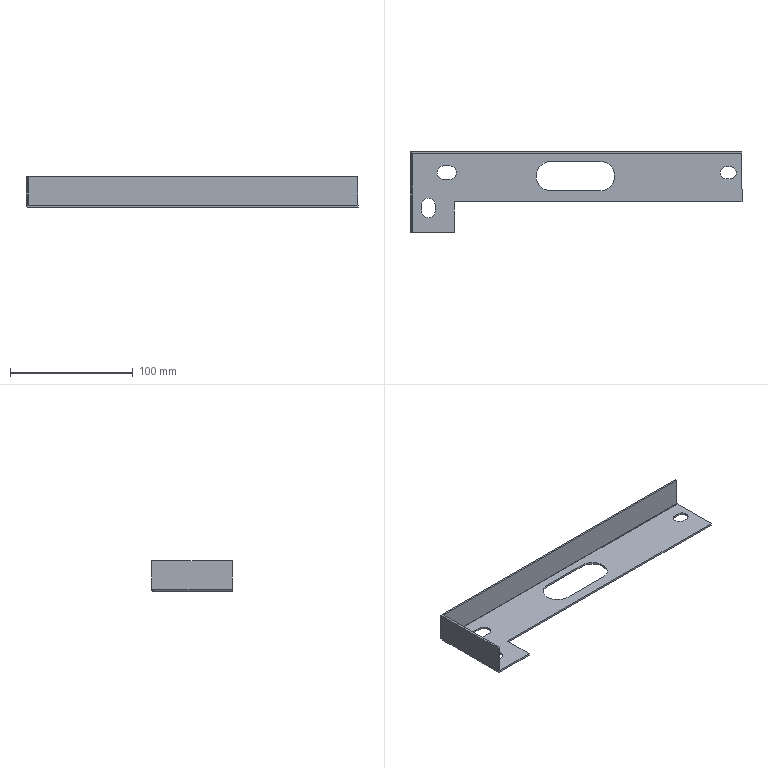Part | 1 solid | 44 faces | box 271 x 66 x 25 mm | volume 26895 mm3 | plane 29 | cylinder 15 | commonest cylinder face diameters 11 x5 10 x3 24 x3 0.4 x2 3.4 x2
STEP:
#1=CARTESIAN_POINT('',(130.8,15.8,-1.5));
#2=VERTEX_POINT('',#1);
#3=CARTESIAN_POINT('',(125.8,20.8,-1.5));
#4=VERTEX_POINT('',#3);
#5=CARTESIAN_POINT('',(125.8,15.8,-1.5));
#6=DIRECTION('',(0.,0.,1.));
#7=DIRECTION('',(1.,0.,0.));
#8=AXIS2_PLACEMENT_3D('',#5,#6,#7);
#9=CIRCLE('',#8,5.);
#10=EDGE_CURVE('',#2,#4,#9,.T.);
#11=ORIENTED_EDGE('',*,*,#10,.F.);
#12=CARTESIAN_POINT('',(130.8,15.8,0.));
#13=VERTEX_POINT('',#12);
#14=CARTESIAN_POINT('',(130.8,15.8,-10.));
#15=DIRECTION('',(0.,0.,1.));
#16=VECTOR('',#15,1000.);
#17=LINE('',#14,#16);
#18=EDGE_CURVE('',#2,#13,#17,.T.);
#19=ORIENTED_EDGE('',*,*,#18,.T.);
#20=CARTESIAN_POINT('',(125.8,20.8,0.));
#21=VERTEX_POINT('',#20);
#22=CARTESIAN_POINT('',(125.8,15.8,0.));
#23=DIRECTION('',(0.,0.,1.));
#24=DIRECTION('',(1.,0.,0.));
#25=AXIS2_PLACEMENT_3D('',#22,#23,#24);
#26=CIRCLE('',#25,5.);
#27=EDGE_CURVE('',#13,#21,#26,.T.);
#28=ORIENTED_EDGE('',*,*,#27,.T.);
#29=CARTESIAN_POINT('',(125.8,20.8,-10.));
#30=DIRECTION('',(0.,0.,1.));
#31=VECTOR('',#30,1000.);
#32=LINE('',#29,#31);
#33=EDGE_CURVE('',#4,#21,#32,.T.);
#34=ORIENTED_EDGE('',*,*,#33,.F.);
#35=EDGE_LOOP('',(#11,#19,#28,#34));
#36=FACE_OUTER_BOUND('',#35,.T.);
#37=CARTESIAN_POINT('',(125.8,15.8,-10.));
#38=DIRECTION('',(0.,0.,1.));
#39=DIRECTION('',(1.,0.,0.));
#40=AXIS2_PLACEMENT_3D('',#37,#38,#39);
#41=CYLINDRICAL_SURFACE('',#40,5.);
#42=ADVANCED_FACE('',(#36),#41,.F.);
#43=CARTESIAN_POINT('',(-97.5,15.8,-1.5));
#44=VERTEX_POINT('',#43);
#45=CARTESIAN_POINT('',(-103.,21.3,-1.5));
#46=VERTEX_POINT('',#45);
#47=CARTESIAN_POINT('',(-103.,15.8,-1.5));
#48=DIRECTION('',(0.,0.,1.));
#49=DIRECTION('',(1.,0.,0.));
#50=AXIS2_PLACEMENT_3D('',#47,#48,#49);
#51=CIRCLE('',#50,5.5);
#52=EDGE_CURVE('',#44,#46,#51,.T.);
#53=ORIENTED_EDGE('',*,*,#52,.F.);
#54=CARTESIAN_POINT('',(-97.5,15.8,0.));
#55=VERTEX_POINT('',#54);
#56=CARTESIAN_POINT('',(-97.5,15.8,-10.));
#57=DIRECTION('',(0.,0.,1.));
#58=VECTOR('',#57,1000.);
#59=LINE('',#56,#58);
#60=EDGE_CURVE('',#44,#55,#59,.T.);
#61=ORIENTED_EDGE('',*,*,#60,.T.);
#62=CARTESIAN_POINT('',(-103.,21.3,0.));
#63=VERTEX_POINT('',#62);
#64=CARTESIAN_POINT('',(-103.,15.8,0.));
#65=DIRECTION('',(0.,0.,1.));
#66=DIRECTION('',(1.,0.,0.));
#67=AXIS2_PLACEMENT_3D('',#64,#65,#66);
#68=CIRCLE('',#67,5.5);
#69=EDGE_CURVE('',#55,#63,#68,.T.);
#70=ORIENTED_EDGE('',*,*,#69,.T.);
#71=CARTESIAN_POINT('',(-103.,21.3,-10.));
#72=DIRECTION('',(0.,0.,1.));
#73=VECTOR('',#72,1000.);
#74=LINE('',#71,#73);
#75=EDGE_CURVE('',#46,#63,#74,.T.);
#76=ORIENTED_EDGE('',*,*,#75,.F.);
#77=EDGE_LOOP('',(#53,#61,#70,#76));
#78=FACE_OUTER_BOUND('',#77,.T.);
#79=CARTESIAN_POINT('',(-103.,15.8,-10.));
#80=DIRECTION('',(0.,0.,1.));
#81=DIRECTION('',(1.,0.,0.));
#82=AXIS2_PLACEMENT_3D('',#79,#80,#81);
#83=CYLINDRICAL_SURFACE('',#82,5.5);
#84=ADVANCED_FACE('',(#78),#83,.F.);
#85=CARTESIAN_POINT('',(31.5,13.,-1.5));
#86=VERTEX_POINT('',#85);
#87=CARTESIAN_POINT('',(19.5,25.,-1.5));
#88=VERTEX_POINT('',#87);
#89=CARTESIAN_POINT('',(19.5,13.,-1.5));
#90=DIRECTION('',(0.,0.,1.));
#91=DIRECTION('',(1.,0.,0.));
#92=AXIS2_PLACEMENT_3D('',#89,#90,#91);
#93=CIRCLE('',#92,12.);
#94=EDGE_CURVE('',#86,#88,#93,.T.);
#95=ORIENTED_EDGE('',*,*,#94,.F.);
#96=CARTESIAN_POINT('',(31.5,13.,0.));
#97=VERTEX_POINT('',#96);
#98=CARTESIAN_POINT('',(31.5,13.,-10.));
#99=DIRECTION('',(0.,0.,1.));
#100=VECTOR('',#99,1000.);
#101=LINE('',#98,#100);
#102=EDGE_CURVE('',#86,#97,#101,.T.);
#103=ORIENTED_EDGE('',*,*,#102,.T.);
#104=CARTESIAN_POINT('',(19.5,25.,0.));
#105=VERTEX_POINT('',#104);
#106=CARTESIAN_POINT('',(19.5,13.,0.));
#107=DIRECTION('',(0.,0.,1.));
#108=DIRECTION('',(1.,0.,0.));
#109=AXIS2_PLACEMENT_3D('',#106,#107,#108);
#110=CIRCLE('',#109,12.);
#111=EDGE_CURVE('',#97,#105,#110,.T.);
#112=ORIENTED_EDGE('',*,*,#111,.T.);
#113=CARTESIAN_POINT('',(19.5,25.,-10.));
#114=DIRECTION('',(0.,0.,1.));
#115=VECTOR('',#114,1000.);
#116=LINE('',#113,#115);
#117=EDGE_CURVE('',#88,#105,#116,.T.);
#118=ORIENTED_EDGE('',*,*,#117,.F.);
#119=EDGE_LOOP('',(#95,#103,#112,#118));
#120=FACE_OUTER_BOUND('',#119,.T.);
#121=CARTESIAN_POINT('',(19.5,13.,-10.));
#122=DIRECTION('',(0.,0.,1.));
#123=DIRECTION('',(1.,0.,0.));
#124=AXIS2_PLACEMENT_3D('',#121,#122,#123);
#125=CYLINDRICAL_SURFACE('',#124,12.);
#126=ADVANCED_FACE('',(#120),#125,.F.);
#127=CARTESIAN_POINT('',(-135.5,31.3,0.2));
#128=VERTEX_POINT('',#127);
#129=CARTESIAN_POINT('',(-134.,31.3,0.2));
#130=VERTEX_POINT('',#129);
#131=CARTESIAN_POINT('',(-135.5,31.3,0.2));
#132=DIRECTION('',(1.,0.,0.));
#133=VECTOR('',#132,1000.);
#134=LINE('',#131,#133);
#135=EDGE_CURVE('',#128,#130,#134,.T.);
#136=ORIENTED_EDGE('',*,*,#135,.F.);
#137=CARTESIAN_POINT('',(-135.5,33.,0.2));
#138=VERTEX_POINT('',#137);
#139=CARTESIAN_POINT('',(-135.5,33.,0.2));
#140=DIRECTION('',(0.,1.,0.));
#141=VECTOR('',#140,1000.);
#142=LINE('',#139,#141);
#143=EDGE_CURVE('',#128,#138,#142,.T.);
#144=ORIENTED_EDGE('',*,*,#143,.T.);
#145=CARTESIAN_POINT('',(-134.,33.,0.2));
#146=VERTEX_POINT('',#145);
#147=CARTESIAN_POINT('',(-135.5,33.,0.2));
#148=DIRECTION('',(-1.,0.,0.));
#149=VECTOR('',#148,1000.);
#150=LINE('',#147,#149);
#151=EDGE_CURVE('',#146,#138,#150,.T.);
#152=ORIENTED_EDGE('',*,*,#151,.F.);
#153=CARTESIAN_POINT('',(-134.,33.,0.2));
#154=DIRECTION('',(0.,-1.,0.));
#155=VECTOR('',#154,1000.);
#156=LINE('',#153,#155);
#157=EDGE_CURVE('',#146,#130,#156,.T.);
#158=ORIENTED_EDGE('',*,*,#157,.T.);
#159=EDGE_LOOP('',(#136,#144,#152,#158));
#160=FACE_OUTER_BOUND('',#159,.T.);
#161=CARTESIAN_POINT('',(0.,0.,0.2));
#162=DIRECTION('',(0.,0.,-1.));
#163=DIRECTION('',(-1.,0.,0.));
#164=AXIS2_PLACEMENT_3D('',#161,#162,#163);
#165=PLANE('',#164);
#166=ADVANCED_FACE('',(#160),#165,.T.);
#167=CARTESIAN_POINT('',(-135.5,-33.,0.2));
#168=VERTEX_POINT('',#167);
#169=CARTESIAN_POINT('',(-135.5,33.,0.2));
#170=DIRECTION('',(0.,1.,0.));
#171=VECTOR('',#170,1000.);
#172=LINE('',#169,#171);
#173=EDGE_CURVE('',#168,#128,#172,.T.);
#174=ORIENTED_EDGE('',*,*,#173,.T.);
#175=CARTESIAN_POINT('',(-133.8,31.3,-1.5));
#176=VERTEX_POINT('',#175);
#177=CARTESIAN_POINT('',(-133.8,31.3,0.2));
#178=DIRECTION('',(0.,-1.,0.));
#179=DIRECTION('',(0.,0.,1.));
#180=AXIS2_PLACEMENT_3D('',#177,#178,#179);
#181=CIRCLE('',#180,1.7);
#182=EDGE_CURVE('',#128,#176,#181,.T.);
#183=ORIENTED_EDGE('',*,*,#182,.T.);
#184=CARTESIAN_POINT('',(-133.8,-33.,-1.5));
#185=VERTEX_POINT('',#184);
#186=CARTESIAN_POINT('',(-133.8,-33.,-1.5));
#187=DIRECTION('',(0.,1.,0.));
#188=VECTOR('',#187,1000.);
#189=LINE('',#186,#188);
#190=EDGE_CURVE('',#185,#176,#189,.T.);
#191=ORIENTED_EDGE('',*,*,#190,.F.);
#192=CARTESIAN_POINT('',(-133.8,-33.,0.2));
#193=DIRECTION('',(0.,-1.,0.));
#194=DIRECTION('',(0.,0.,-1.));
#195=AXIS2_PLACEMENT_3D('',#192,#193,#194);
#196=CIRCLE('',#195,1.7);
#197=EDGE_CURVE('',#168,#185,#196,.T.);
#198=ORIENTED_EDGE('',*,*,#197,.F.);
#199=EDGE_LOOP('',(#174,#183,#191,#198));
#200=FACE_OUTER_BOUND('',#199,.T.);
#201=CARTESIAN_POINT('',(-133.8,-33.,0.2));
#202=DIRECTION('',(0.,-1.,0.));
#203=DIRECTION('',(-1.,0.,0.));
#204=AXIS2_PLACEMENT_3D('',#201,#202,#203);
#205=CYLINDRICAL_SURFACE('',#204,1.7);
#206=ADVANCED_FACE('',(#200),#205,.T.);
#207=CARTESIAN_POINT('',(122.8,20.8,-1.5));
#208=VERTEX_POINT('',#207);
#209=CARTESIAN_POINT('',(0.,20.8,-1.5));
#210=DIRECTION('',(-1.,0.,0.));
#211=VECTOR('',#210,1000.);
#212=LINE('',#209,#211);
#213=EDGE_CURVE('',#4,#208,#212,.T.);
#214=ORIENTED_EDGE('',*,*,#213,.T.);
#215=CARTESIAN_POINT('',(122.8,10.8,-1.5));
#216=VERTEX_POINT('',#215);
#217=CARTESIAN_POINT('',(122.8,15.8,-1.5));
#218=DIRECTION('',(0.,0.,1.));
#219=DIRECTION('',(1.,0.,0.));
#220=AXIS2_PLACEMENT_3D('',#217,#218,#219);
#221=CIRCLE('',#220,5.);
#222=EDGE_CURVE('',#208,#216,#221,.T.);
#223=ORIENTED_EDGE('',*,*,#222,.T.);
#224=CARTESIAN_POINT('',(125.8,10.8,-1.5));
#225=VERTEX_POINT('',#224);
#226=CARTESIAN_POINT('',(0.,10.8,-1.5));
#227=DIRECTION('',(1.,0.,0.));
#228=VECTOR('',#227,1000.);
#229=LINE('',#226,#228);
#230=EDGE_CURVE('',#216,#225,#229,.T.);
#231=ORIENTED_EDGE('',*,*,#230,.T.);
#232=CARTESIAN_POINT('',(125.8,15.8,-1.5));
#233=DIRECTION('',(0.,0.,1.));
#234=DIRECTION('',(1.,0.,0.));
#235=AXIS2_PLACEMENT_3D('',#232,#233,#234);
#236=CIRCLE('',#235,5.);
#237=EDGE_CURVE('',#225,#2,#236,.T.);
#238=ORIENTED_EDGE('',*,*,#237,.T.);
#239=ORIENTED_EDGE('',*,*,#10,.T.);
#240=EDGE_LOOP('',(#214,#223,#231,#238,#239));
#241=FACE_BOUND('',#240,.T.);
#242=CARTESIAN_POINT('',(-108.,21.3,-1.5));
#243=VERTEX_POINT('',#242);
#244=CARTESIAN_POINT('',(0.,21.3,-1.5));
#245=DIRECTION('',(-1.,0.,0.));
#246=VECTOR('',#245,1000.);
#247=LINE('',#244,#246);
#248=EDGE_CURVE('',#46,#243,#247,.T.);
#249=ORIENTED_EDGE('',*,*,#248,.T.);
#250=CARTESIAN_POINT('',(-108.,10.3,-1.5));
#251=VERTEX_POINT('',#250);
#252=CARTESIAN_POINT('',(-108.,15.8,-1.5));
#253=DIRECTION('',(0.,0.,1.));
#254=DIRECTION('',(1.,0.,0.));
#255=AXIS2_PLACEMENT_3D('',#252,#253,#254);
#256=CIRCLE('',#255,5.5);
#257=EDGE_CURVE('',#243,#251,#256,.T.);
#258=ORIENTED_EDGE('',*,*,#257,.T.);
#259=CARTESIAN_POINT('',(-103.,10.3,-1.5));
#260=VERTEX_POINT('',#259);
#261=CARTESIAN_POINT('',(0.,10.3,-1.5));
#262=DIRECTION('',(1.,0.,0.));
#263=VECTOR('',#262,1000.);
#264=LINE('',#261,#263);
#265=EDGE_CURVE('',#251,#260,#264,.T.);
#266=ORIENTED_EDGE('',*,*,#265,.T.);
#267=CARTESIAN_POINT('',(-103.,15.8,-1.5));
#268=DIRECTION('',(0.,0.,1.));
#269=DIRECTION('',(1.,0.,0.));
#270=AXIS2_PLACEMENT_3D('',#267,#268,#269);
#271=CIRCLE('',#270,5.5);
#272=EDGE_CURVE('',#260,#44,#271,.T.);
#273=ORIENTED_EDGE('',*,*,#272,.T.);
#274=ORIENTED_EDGE('',*,*,#52,.T.);
#275=EDGE_LOOP('',(#249,#258,#266,#273,#274));
#276=FACE_BOUND('',#275,.T.);
#277=CARTESIAN_POINT('',(-20.5,25.,-1.5));
#278=VERTEX_POINT('',#277);
#279=CARTESIAN_POINT('',(0.,25.,-1.5));
#280=DIRECTION('',(-1.,0.,0.));
#281=VECTOR('',#280,1000.);
#282=LINE('',#279,#281);
#283=EDGE_CURVE('',#88,#278,#282,.T.);
#284=ORIENTED_EDGE('',*,*,#283,.T.);
#285=CARTESIAN_POINT('',(-20.5,1.,-1.5));
#286=VERTEX_POINT('',#285);
#287=CARTESIAN_POINT('',(-20.5,13.,-1.5));
#288=DIRECTION('',(0.,0.,1.));
#289=DIRECTION('',(1.,0.,0.));
#290=AXIS2_PLACEMENT_3D('',#287,#288,#289);
#291=CIRCLE('',#290,12.);
#292=EDGE_CURVE('',#278,#286,#291,.T.);
#293=ORIENTED_EDGE('',*,*,#292,.T.);
#294=CARTESIAN_POINT('',(19.5,1.,-1.5));
#295=VERTEX_POINT('',#294);
#296=CARTESIAN_POINT('',(0.,1.,-1.5));
#297=DIRECTION('',(1.,0.,0.));
#298=VECTOR('',#297,1000.);
#299=LINE('',#296,#298);
#300=EDGE_CURVE('',#286,#295,#299,.T.);
#301=ORIENTED_EDGE('',*,*,#300,.T.);
#302=CARTESIAN_POINT('',(19.5,13.,-1.5));
#303=DIRECTION('',(0.,0.,1.));
#304=DIRECTION('',(1.,0.,0.));
#305=AXIS2_PLACEMENT_3D('',#302,#303,#304);
#306=CIRCLE('',#305,12.);
#307=EDGE_CURVE('',#295,#86,#306,.T.);
#308=ORIENTED_EDGE('',*,*,#307,.T.);
#309=ORIENTED_EDGE('',*,*,#94,.T.);
#310=EDGE_LOOP('',(#284,#293,#301,#308,#309));
#311=FACE_BOUND('',#310,.T.);
#312=CARTESIAN_POINT('',(-115.,-15.5,-1.5));
#313=VERTEX_POINT('',#312);
#314=CARTESIAN_POINT('',(-115.,-10.5,-1.5));
#315=VERTEX_POINT('',#314);
#316=CARTESIAN_POINT('',(-115.,0.,-1.5));
#317=DIRECTION('',(0.,1.,0.));
#318=VECTOR('',#317,1000.);
#319=LINE('',#316,#318);
#320=EDGE_CURVE('',#313,#315,#319,.T.);
#321=ORIENTED_EDGE('',*,*,#320,.T.);
#322=CARTESIAN_POINT('',(-126.,-10.5,-1.5));
#323=VERTEX_POINT('',#322);
#324=CARTESIAN_POINT('',(-120.5,-10.5,-1.5));
#325=DIRECTION('',(0.,0.,1.));
#326=DIRECTION('',(1.,0.,0.));
#327=AXIS2_PLACEMENT_3D('',#324,#325,#326);
#328=CIRCLE('',#327,5.5);
#329=EDGE_CURVE('',#315,#323,#328,.T.);
#330=ORIENTED_EDGE('',*,*,#329,.T.);
#331=CARTESIAN_POINT('',(-126.,-15.5,-1.5));
#332=VERTEX_POINT('',#331);
#333=CARTESIAN_POINT('',(-126.,0.,-1.5));
#334=DIRECTION('',(0.,-1.,0.));
#335=VECTOR('',#334,1000.);
#336=LINE('',#333,#335);
#337=EDGE_CURVE('',#323,#332,#336,.T.);
#338=ORIENTED_EDGE('',*,*,#337,.T.);
#339=CARTESIAN_POINT('',(-120.5,-15.5,-1.5));
#340=DIRECTION('',(0.,0.,1.));
#341=DIRECTION('',(1.,0.,0.));
#342=AXIS2_PLACEMENT_3D('',#339,#340,#341);
#343=CIRCLE('',#342,5.5);
#344=EDGE_CURVE('',#332,#313,#343,.T.);
#345=ORIENTED_EDGE('',*,*,#344,.T.);
#346=EDGE_LOOP('',(#321,#330,#338,#345));
#347=FACE_BOUND('',#346,.T.);
#348=CARTESIAN_POINT('',(135.5,-8.,-1.5));
#349=VERTEX_POINT('',#348);
#350=CARTESIAN_POINT('',(135.5,31.3,-1.5));
#351=VERTEX_POINT('',#350);
#352=CARTESIAN_POINT('',(135.5,33.,-1.5));
#353=DIRECTION('',(0.,1.,0.));
#354=VECTOR('',#353,1000.);
#355=LINE('',#352,#354);
#356=EDGE_CURVE('',#349,#351,#355,.T.);
#357=ORIENTED_EDGE('',*,*,#356,.F.);
#358=CARTESIAN_POINT('',(-99.5,-8.,-1.5));
#359=VERTEX_POINT('',#358);
#360=CARTESIAN_POINT('',(0.,-8.,-1.5));
#361=DIRECTION('',(-1.,0.,0.));
#362=VECTOR('',#361,1000.);
#363=LINE('',#360,#362);
#364=EDGE_CURVE('',#349,#359,#363,.T.);
#365=ORIENTED_EDGE('',*,*,#364,.T.);
#366=CARTESIAN_POINT('',(-99.5,-33.,-1.5));
#367=VERTEX_POINT('',#366);
#368=CARTESIAN_POINT('',(-99.5,0.,-1.5));
#369=DIRECTION('',(0.,-1.,0.));
#370=VECTOR('',#369,1000.);
#371=LINE('',#368,#370);
#372=EDGE_CURVE('',#359,#367,#371,.T.);
#373=ORIENTED_EDGE('',*,*,#372,.T.);
#374=CARTESIAN_POINT('',(-135.5,-33.,-1.5));
#375=DIRECTION('',(1.,0.,0.));
#376=VECTOR('',#375,1000.);
#377=LINE('',#374,#376);
#378=EDGE_CURVE('',#185,#367,#377,.T.);
#379=ORIENTED_EDGE('',*,*,#378,.F.);
#380=ORIENTED_EDGE('',*,*,#190,.T.);
#381=CARTESIAN_POINT('',(-133.8,31.3,-1.5));
#382=DIRECTION('',(1.,0.,0.));
#383=VECTOR('',#382,1000.);
#384=LINE('',#381,#383);
#385=EDGE_CURVE('',#176,#351,#384,.T.);
#386=ORIENTED_EDGE('',*,*,#385,.T.);
#387=EDGE_LOOP('',(#357,#365,#373,#379,#380,#386));
#388=FACE_OUTER_BOUND('',#387,.T.);
#389=CARTESIAN_POINT('',(0.,0.,-1.5));
#390=DIRECTION('',(0.,0.,1.));
#391=DIRECTION('',(1.,0.,0.));
#392=AXIS2_PLACEMENT_3D('',#389,#390,#391);
#393=PLANE('',#392);
#394=ADVANCED_FACE('',(#241,#276,#311,#347,#388),#393,.F.);
#395=CARTESIAN_POINT('',(135.5,-8.,0.));
#396=VERTEX_POINT('',#395);
#397=CARTESIAN_POINT('',(-99.5,-8.,0.));
#398=VERTEX_POINT('',#397);
#399=CARTESIAN_POINT('',(0.,-8.,0.));
#400=DIRECTION('',(-1.,0.,0.));
#401=VECTOR('',#400,1000.);
#402=LINE('',#399,#401);
#403=EDGE_CURVE('',#396,#398,#402,.T.);
#404=ORIENTED_EDGE('',*,*,#403,.F.);
#405=CARTESIAN_POINT('',(135.5,31.3,0.));
#406=VERTEX_POINT('',#405);
#407=CARTESIAN_POINT('',(135.5,33.,0.));
#408=DIRECTION('',(0.,1.,0.));
#409=VECTOR('',#408,1000.);
#410=LINE('',#407,#409);
#411=EDGE_CURVE('',#396,#406,#410,.T.);
#412=ORIENTED_EDGE('',*,*,#411,.T.);
#413=CARTESIAN_POINT('',(-133.8,31.3,0.));
#414=VERTEX_POINT('',#413);
#415=CARTESIAN_POINT('',(-133.8,31.3,0.));
#416=DIRECTION('',(1.,0.,0.));
#417=VECTOR('',#416,1000.);
#418=LINE('',#415,#417);
#419=EDGE_CURVE('',#414,#406,#418,.T.);
#420=ORIENTED_EDGE('',*,*,#419,.F.);
#421=CARTESIAN_POINT('',(-133.8,-33.,0.));
#422=VERTEX_POINT('',#421);
#423=CARTESIAN_POINT('',(-133.8,-33.,0.));
#424=DIRECTION('',(0.,1.,0.));
#425=VECTOR('',#424,1000.);
#426=LINE('',#423,#425);
#427=EDGE_CURVE('',#422,#414,#426,.T.);
#428=ORIENTED_EDGE('',*,*,#427,.F.);
#429=CARTESIAN_POINT('',(-99.5,-33.,0.));
#430=VERTEX_POINT('',#429);
#431=CARTESIAN_POINT('',(-135.5,-33.,0.));
#432=DIRECTION('',(1.,0.,0.));
#433=VECTOR('',#432,1000.);
#434=LINE('',#431,#433);
#435=EDGE_CURVE('',#422,#430,#434,.T.);
#436=ORIENTED_EDGE('',*,*,#435,.T.);
#437=CARTESIAN_POINT('',(-99.5,0.,0.));
#438=DIRECTION('',(0.,-1.,0.));
#439=VECTOR('',#438,1000.);
#440=LINE('',#437,#439);
#441=EDGE_CURVE('',#398,#430,#440,.T.);
#442=ORIENTED_EDGE('',*,*,#441,.F.);
#443=EDGE_LOOP('',(#404,#412,#420,#428,#436,#442));
#444=FACE_OUTER_BOUND('',#443,.T.);
#445=CARTESIAN_POINT('',(122.8,20.8,0.));
#446=VERTEX_POINT('',#445);
#447=CARTESIAN_POINT('',(122.8,10.8,0.));
#448=VERTEX_POINT('',#447);
#449=CARTESIAN_POINT('',(122.8,15.8,0.));
#450=DIRECTION('',(0.,0.,1.));
#451=DIRECTION('',(1.,0.,0.));
#452=AXIS2_PLACEMENT_3D('',#449,#450,#451);
#453=CIRCLE('',#452,5.);
#454=EDGE_CURVE('',#446,#448,#453,.T.);
#455=ORIENTED_EDGE('',*,*,#454,.F.);
#456=CARTESIAN_POINT('',(122.8,20.8,0.));
#457=DIRECTION('',(-1.,0.,0.));
#458=VECTOR('',#457,1000.);
#459=LINE('',#456,#458);
#460=EDGE_CURVE('',#21,#446,#459,.T.);
#461=ORIENTED_EDGE('',*,*,#460,.F.);
#462=ORIENTED_EDGE('',*,*,#27,.F.);
#463=CARTESIAN_POINT('',(125.8,10.8,0.));
#464=VERTEX_POINT('',#463);
#465=CARTESIAN_POINT('',(125.8,15.8,0.));
#466=DIRECTION('',(0.,0.,1.));
#467=DIRECTION('',(1.,0.,0.));
#468=AXIS2_PLACEMENT_3D('',#465,#466,#467);
#469=CIRCLE('',#468,5.);
#470=EDGE_CURVE('',#464,#13,#469,.T.);
#471=ORIENTED_EDGE('',*,*,#470,.F.);
#472=CARTESIAN_POINT('',(122.8,10.8,0.));
#473=DIRECTION('',(1.,0.,0.));
#474=VECTOR('',#473,1000.);
#475=LINE('',#472,#474);
#476=EDGE_CURVE('',#448,#464,#475,.T.);
#477=ORIENTED_EDGE('',*,*,#476,.F.);
#478=EDGE_LOOP('',(#455,#461,#462,#471,#477));
#479=FACE_BOUND('',#478,.T.);
#480=CARTESIAN_POINT('',(-108.,21.3,0.));
#481=VERTEX_POINT('',#480);
#482=CARTESIAN_POINT('',(-108.,10.3,0.));
#483=VERTEX_POINT('',#482);
#484=CARTESIAN_POINT('',(-108.,15.8,0.));
#485=DIRECTION('',(0.,0.,1.));
#486=DIRECTION('',(1.,0.,0.));
#487=AXIS2_PLACEMENT_3D('',#484,#485,#486);
#488=CIRCLE('',#487,5.5);
#489=EDGE_CURVE('',#481,#483,#488,.T.);
#490=ORIENTED_EDGE('',*,*,#489,.F.);
#491=CARTESIAN_POINT('',(-108.,21.3,0.));
#492=DIRECTION('',(-1.,0.,0.));
#493=VECTOR('',#492,1000.);
#494=LINE('',#491,#493);
#495=EDGE_CURVE('',#63,#481,#494,.T.);
#496=ORIENTED_EDGE('',*,*,#495,.F.);
#497=ORIENTED_EDGE('',*,*,#69,.F.);
#498=CARTESIAN_POINT('',(-103.,10.3,0.));
#499=VERTEX_POINT('',#498);
#500=CARTESIAN_POINT('',(-103.,15.8,0.));
#501=DIRECTION('',(0.,0.,1.));
#502=DIRECTION('',(1.,0.,0.));
#503=AXIS2_PLACEMENT_3D('',#500,#501,#502);
#504=CIRCLE('',#503,5.5);
#505=EDGE_CURVE('',#499,#55,#504,.T.);
#506=ORIENTED_EDGE('',*,*,#505,.F.);
#507=CARTESIAN_POINT('',(-108.,10.3,0.));
#508=DIRECTION('',(1.,0.,0.));
#509=VECTOR('',#508,1000.);
#510=LINE('',#507,#509);
#511=EDGE_CURVE('',#483,#499,#510,.T.);
#512=ORIENTED_EDGE('',*,*,#511,.F.);
#513=EDGE_LOOP('',(#490,#496,#497,#506,#512));
#514=FACE_BOUND('',#513,.T.);
#515=CARTESIAN_POINT('',(-20.5,25.,0.));
#516=VERTEX_POINT('',#515);
#517=CARTESIAN_POINT('',(-20.5,1.,0.));
#518=VERTEX_POINT('',#517);
#519=CARTESIAN_POINT('',(-20.5,13.,0.));
#520=DIRECTION('',(0.,0.,1.));
#521=DIRECTION('',(1.,0.,0.));
#522=AXIS2_PLACEMENT_3D('',#519,#520,#521);
#523=CIRCLE('',#522,12.);
#524=EDGE_CURVE('',#516,#518,#523,.T.);
#525=ORIENTED_EDGE('',*,*,#524,.F.);
#526=CARTESIAN_POINT('',(-20.5,25.,0.));
#527=DIRECTION('',(-1.,0.,0.));
#528=VECTOR('',#527,1000.);
#529=LINE('',#526,#528);
#530=EDGE_CURVE('',#105,#516,#529,.T.);
#531=ORIENTED_EDGE('',*,*,#530,.F.);
#532=ORIENTED_EDGE('',*,*,#111,.F.);
#533=CARTESIAN_POINT('',(19.5,1.,0.));
#534=VERTEX_POINT('',#533);
#535=CARTESIAN_POINT('',(19.5,13.,0.));
#536=DIRECTION('',(0.,0.,1.));
#537=DIRECTION('',(1.,0.,0.));
#538=AXIS2_PLACEMENT_3D('',#535,#536,#537);
#539=CIRCLE('',#538,12.);
#540=EDGE_CURVE('',#534,#97,#539,.T.);
#541=ORIENTED_EDGE('',*,*,#540,.F.);
#542=CARTESIAN_POINT('',(-20.5,1.,0.));
#543=DIRECTION('',(1.,0.,0.));
#544=VECTOR('',#543,1000.);
#545=LINE('',#542,#544);
#546=EDGE_CURVE('',#518,#534,#545,.T.);
#547=ORIENTED_EDGE('',*,*,#546,.F.);
#548=EDGE_LOOP('',(#525,#531,#532,#541,#547));
#549=FACE_BOUND('',#548,.T.);
#550=CARTESIAN_POINT('',(-115.,-10.5,0.));
#551=VERTEX_POINT('',#550);
#552=CARTESIAN_POINT('',(-126.,-10.5,0.));
#553=VERTEX_POINT('',#552);
#554=CARTESIAN_POINT('',(-120.5,-10.5,0.));
#555=DIRECTION('',(0.,0.,1.));
#556=DIRECTION('',(1.,0.,0.));
#557=AXIS2_PLACEMENT_3D('',#554,#555,#556);
#558=CIRCLE('',#557,5.5);
#559=EDGE_CURVE('',#551,#553,#558,.T.);
#560=ORIENTED_EDGE('',*,*,#559,.F.);
#561=CARTESIAN_POINT('',(-115.,-15.5,0.));
#562=VERTEX_POINT('',#561);
#563=CARTESIAN_POINT('',(-115.,-10.5,0.));
#564=DIRECTION('',(0.,1.,0.));
#565=VECTOR('',#564,1000.);
#566=LINE('',#563,#565);
#567=EDGE_CURVE('',#562,#551,#566,.T.);
#568=ORIENTED_EDGE('',*,*,#567,.F.);
#569=CARTESIAN_POINT('',(-126.,-15.5,0.));
#570=VERTEX_POINT('',#569);
#571=CARTESIAN_POINT('',(-120.5,-15.5,0.));
#572=DIRECTION('',(0.,0.,1.));
#573=DIRECTION('',(1.,0.,0.));
#574=AXIS2_PLACEMENT_3D('',#571,#572,#573);
#575=CIRCLE('',#574,5.5);
#576=EDGE_CURVE('',#570,#562,#575,.T.);
#577=ORIENTED_EDGE('',*,*,#576,.F.);
#578=CARTESIAN_POINT('',(-126.,-10.5,0.));
#579=DIRECTION('',(0.,-1.,0.));
#580=VECTOR('',#579,1000.);
#581=LINE('',#578,#580);
#582=EDGE_CURVE('',#553,#570,#581,.T.);
#583=ORIENTED_EDGE('',*,*,#582,.F.);
#584=EDGE_LOOP('',(#560,#568,#577,#583));
#585=FACE_BOUND('',#584,.T.);
#586=CARTESIAN_POINT('',(0.,0.,0.));
#587=DIRECTION('',(0.,0.,1.));
#588=DIRECTION('',(1.,0.,0.));
#589=AXIS2_PLACEMENT_3D('',#586,#587,#588);
#590=PLANE('',#589);
#591=ADVANCED_FACE('',(#444,#479,#514,#549,#585),#590,.T.);
#592=CARTESIAN_POINT('',(-99.5,-33.,23.5));
#593=DIRECTION('',(0.,0.,-1.));
#594=VECTOR('',#593,1000.);
#595=LINE('',#592,#594);
#596=EDGE_CURVE('',#430,#367,#595,.T.);
#597=ORIENTED_EDGE('',*,*,#596,.F.);
#598=ORIENTED_EDGE('',*,*,#435,.F.);
#599=CARTESIAN_POINT('',(-133.8,-33.,0.));
#600=DIRECTION('',(0.,0.,-1.));
#601=VECTOR('',#600,1000.);
#602=LINE('',#599,#601);
#603=EDGE_CURVE('',#422,#185,#602,.T.);
#604=ORIENTED_EDGE('',*,*,#603,.T.);
#605=ORIENTED_EDGE('',*,*,#378,.T.);
#606=EDGE_LOOP('',(#597,#598,#604,#605));
#607=FACE_OUTER_BOUND('',#606,.T.);
#608=CARTESIAN_POINT('',(-135.5,-33.,-1.5));
#609=DIRECTION('',(0.,-1.,0.));
#610=DIRECTION('',(0.,0.,-1.));
#611=AXIS2_PLACEMENT_3D('',#608,#609,#610);
#612=PLANE('',#611);
#613=ADVANCED_FACE('',(#607),#612,.T.);
#614=CARTESIAN_POINT('',(135.5,-8.,-1.5));
#615=DIRECTION('',(0.,0.,1.));
#616=VECTOR('',#615,1000.);
#617=LINE('',#614,#616);
#618=EDGE_CURVE('',#349,#396,#617,.T.);
#619=ORIENTED_EDGE('',*,*,#618,.F.);
#620=ORIENTED_EDGE('',*,*,#356,.T.);
#621=CARTESIAN_POINT('',(135.5,31.3,0.));
#622=DIRECTION('',(0.,0.,-1.));
#623=VECTOR('',#622,1000.);
#624=LINE('',#621,#623);
#625=EDGE_CURVE('',#406,#351,#624,.T.);
#626=ORIENTED_EDGE('',*,*,#625,.F.);
#627=ORIENTED_EDGE('',*,*,#411,.F.);
#628=EDGE_LOOP('',(#619,#620,#626,#627));
#629=FACE_OUTER_BOUND('',#628,.T.);
#630=CARTESIAN_POINT('',(135.5,33.,-1.5));
#631=DIRECTION('',(1.,0.,0.));
#632=DIRECTION('',(0.,0.,-1.));
#633=AXIS2_PLACEMENT_3D('',#630,#631,#632);
#634=PLANE('',#633);
#635=ADVANCED_FACE('',(#629),#634,.T.);
#636=CARTESIAN_POINT('',(-115.,-10.5,-10.));
#637=DIRECTION('',(0.,0.,1.));
#638=VECTOR('',#637,1000.);
#639=LINE('',#636,#638);
#640=EDGE_CURVE('',#315,#551,#639,.T.);
#641=ORIENTED_EDGE('',*,*,#640,.T.);
#642=ORIENTED_EDGE('',*,*,#559,.T.);
#643=CARTESIAN_POINT('',(-126.,-10.5,-10.));
#644=DIRECTION('',(0.,0.,1.));
#645=VECTOR('',#644,1000.);
#646=LINE('',#643,#645);
#647=EDGE_CURVE('',#323,#553,#646,.T.);
#648=ORIENTED_EDGE('',*,*,#647,.F.);
#649=ORIENTED_EDGE('',*,*,#329,.F.);
#650=EDGE_LOOP('',(#641,#642,#648,#649));
#651=FACE_OUTER_BOUND('',#650,.T.);
#652=CARTESIAN_POINT('',(-120.5,-10.5,-10.));
#653=DIRECTION('',(0.,0.,1.));
#654=DIRECTION('',(1.,0.,0.));
#655=AXIS2_PLACEMENT_3D('',#652,#653,#654);
#656=CYLINDRICAL_SURFACE('',#655,5.5);
#657=ADVANCED_FACE('',(#651),#656,.F.);
#658=CARTESIAN_POINT('',(-115.,-15.5,-10.));
#659=DIRECTION('',(0.,0.,1.));
#660=VECTOR('',#659,1000.);
#661=LINE('',#658,#660);
#662=EDGE_CURVE('',#313,#562,#661,.T.);
#663=ORIENTED_EDGE('',*,*,#662,.T.);
#664=ORIENTED_EDGE('',*,*,#567,.T.);
#665=ORIENTED_EDGE('',*,*,#640,.F.);
#666=ORIENTED_EDGE('',*,*,#320,.F.);
#667=EDGE_LOOP('',(#663,#664,#665,#666));
#668=FACE_OUTER_BOUND('',#667,.T.);
#669=CARTESIAN_POINT('',(-115.,-10.5,-10.));
#670=DIRECTION('',(1.,0.,0.));
#671=DIRECTION('',(0.,0.,-1.));
#672=AXIS2_PLACEMENT_3D('',#669,#670,#671);
#673=PLANE('',#672);
#674=ADVANCED_FACE('',(#668),#673,.F.);
#675=CARTESIAN_POINT('',(-126.,-15.5,-10.));
#676=DIRECTION('',(0.,0.,1.));
#677=VECTOR('',#676,1000.);
#678=LINE('',#675,#677);
#679=EDGE_CURVE('',#332,#570,#678,.T.);
#680=ORIENTED_EDGE('',*,*,#679,.T.);
#681=ORIENTED_EDGE('',*,*,#576,.T.);
#682=ORIENTED_EDGE('',*,*,#662,.F.);
#683=ORIENTED_EDGE('',*,*,#344,.F.);
#684=EDGE_LOOP('',(#680,#681,#682,#683));
#685=FACE_OUTER_BOUND('',#684,.T.);
#686=CARTESIAN_POINT('',(-120.5,-15.5,-10.));
#687=DIRECTION('',(0.,0.,1.));
#688=DIRECTION('',(1.,0.,0.));
#689=AXIS2_PLACEMENT_3D('',#686,#687,#688);
#690=CYLINDRICAL_SURFACE('',#689,5.5);
#691=ADVANCED_FACE('',(#685),#690,.F.);
#692=ORIENTED_EDGE('',*,*,#647,.T.);
#693=ORIENTED_EDGE('',*,*,#582,.T.);
#694=ORIENTED_EDGE('',*,*,#679,.F.);
#695=ORIENTED_EDGE('',*,*,#337,.F.);
#696=EDGE_LOOP('',(#692,#693,#694,#695));
#697=FACE_OUTER_BOUND('',#696,.T.);
#698=CARTESIAN_POINT('',(-126.,-10.5,-10.));
#699=DIRECTION('',(-1.,0.,0.));
#700=DIRECTION('',(0.,0.,1.));
#701=AXIS2_PLACEMENT_3D('',#698,#699,#700);
#702=PLANE('',#701);
#703=ADVANCED_FACE('',(#697),#702,.F.);
#704=CARTESIAN_POINT('',(-20.5,25.,-10.));
#705=DIRECTION('',(0.,0.,1.));
#706=VECTOR('',#705,1000.);
#707=LINE('',#704,#706);
#708=EDGE_CURVE('',#278,#516,#707,.T.);
#709=ORIENTED_EDGE('',*,*,#708,.T.);
#710=ORIENTED_EDGE('',*,*,#524,.T.);
#711=CARTESIAN_POINT('',(-20.5,1.,-10.));
#712=DIRECTION('',(0.,0.,1.));
#713=VECTOR('',#712,1000.);
#714=LINE('',#711,#713);
#715=EDGE_CURVE('',#286,#518,#714,.T.);
#716=ORIENTED_EDGE('',*,*,#715,.F.);
#717=ORIENTED_EDGE('',*,*,#292,.F.);
#718=EDGE_LOOP('',(#709,#710,#716,#717));
#719=FACE_OUTER_BOUND('',#718,.T.);
#720=CARTESIAN_POINT('',(-20.5,13.,-10.));
#721=DIRECTION('',(0.,0.,1.));
#722=DIRECTION('',(1.,0.,0.));
#723=AXIS2_PLACEMENT_3D('',#720,#721,#722);
#724=CYLINDRICAL_SURFACE('',#723,12.);
#725=ADVANCED_FACE('',(#719),#724,.F.);
#726=ORIENTED_EDGE('',*,*,#117,.T.);
#727=ORIENTED_EDGE('',*,*,#530,.T.);
#728=ORIENTED_EDGE('',*,*,#708,.F.);
#729=ORIENTED_EDGE('',*,*,#283,.F.);
#730=EDGE_LOOP('',(#726,#727,#728,#729));
#731=FACE_OUTER_BOUND('',#730,.T.);
#732=CARTESIAN_POINT('',(-20.5,25.,-10.));
#733=DIRECTION('',(0.,1.,0.));
#734=DIRECTION('',(-1.,0.,0.));
#735=AXIS2_PLACEMENT_3D('',#732,#733,#734);
#736=PLANE('',#735);
#737=ADVANCED_FACE('',(#731),#736,.F.);
#738=ORIENTED_EDGE('',*,*,#102,.F.);
#739=ORIENTED_EDGE('',*,*,#307,.F.);
#740=CARTESIAN_POINT('',(19.5,1.,-10.));
#741=DIRECTION('',(0.,0.,1.));
#742=VECTOR('',#741,1000.);
#743=LINE('',#740,#742);
#744=EDGE_CURVE('',#295,#534,#743,.T.);
#745=ORIENTED_EDGE('',*,*,#744,.T.);
#746=ORIENTED_EDGE('',*,*,#540,.T.);
#747=EDGE_LOOP('',(#738,#739,#745,#746));
#748=FACE_OUTER_BOUND('',#747,.T.);
#749=CARTESIAN_POINT('',(19.5,13.,-10.));
#750=DIRECTION('',(0.,0.,1.));
#751=DIRECTION('',(1.,0.,0.));
#752=AXIS2_PLACEMENT_3D('',#749,#750,#751);
#753=CYLINDRICAL_SURFACE('',#752,12.);
#754=ADVANCED_FACE('',(#748),#753,.F.);
#755=ORIENTED_EDGE('',*,*,#715,.T.);
#756=ORIENTED_EDGE('',*,*,#546,.T.);
#757=ORIENTED_EDGE('',*,*,#744,.F.);
#758=ORIENTED_EDGE('',*,*,#300,.F.);
#759=EDGE_LOOP('',(#755,#756,#757,#758));
#760=FACE_OUTER_BOUND('',#759,.T.);
#761=CARTESIAN_POINT('',(-20.5,1.,-10.));
#762=DIRECTION('',(0.,-1.,0.));
#763=DIRECTION('',(1.,0.,0.));
#764=AXIS2_PLACEMENT_3D('',#761,#762,#763);
#765=PLANE('',#764);
#766=ADVANCED_FACE('',(#760),#765,.F.);
#767=CARTESIAN_POINT('',(-108.,21.3,-10.));
#768=DIRECTION('',(0.,0.,1.));
#769=VECTOR('',#768,1000.);
#770=LINE('',#767,#769);
#771=EDGE_CURVE('',#243,#481,#770,.T.);
#772=ORIENTED_EDGE('',*,*,#771,.T.);
#773=ORIENTED_EDGE('',*,*,#489,.T.);
#774=CARTESIAN_POINT('',(-108.,10.3,-10.));
#775=DIRECTION('',(0.,0.,1.));
#776=VECTOR('',#775,1000.);
#777=LINE('',#774,#776);
#778=EDGE_CURVE('',#251,#483,#777,.T.);
#779=ORIENTED_EDGE('',*,*,#778,.F.);
#780=ORIENTED_EDGE('',*,*,#257,.F.);
#781=EDGE_LOOP('',(#772,#773,#779,#780));
#782=FACE_OUTER_BOUND('',#781,.T.);
#783=CARTESIAN_POINT('',(-108.,15.8,-10.));
#784=DIRECTION('',(0.,0.,1.));
#785=DIRECTION('',(1.,0.,0.));
#786=AXIS2_PLACEMENT_3D('',#783,#784,#785);
#787=CYLINDRICAL_SURFACE('',#786,5.5);
#788=ADVANCED_FACE('',(#782),#787,.F.);
#789=ORIENTED_EDGE('',*,*,#75,.T.);
#790=ORIENTED_EDGE('',*,*,#495,.T.);
#791=ORIENTED_EDGE('',*,*,#771,.F.);
#792=ORIENTED_EDGE('',*,*,#248,.F.);
#793=EDGE_LOOP('',(#789,#790,#791,#792));
#794=FACE_OUTER_BOUND('',#793,.T.);
#795=CARTESIAN_POINT('',(-108.,21.3,-10.));
#796=DIRECTION('',(0.,1.,0.));
#797=DIRECTION('',(0.,0.,1.));
#798=AXIS2_PLACEMENT_3D('',#795,#796,#797);
#799=PLANE('',#798);
#800=ADVANCED_FACE('',(#794),#799,.F.);
#801=ORIENTED_EDGE('',*,*,#60,.F.);
#802=ORIENTED_EDGE('',*,*,#272,.F.);
#803=CARTESIAN_POINT('',(-103.,10.3,-10.));
#804=DIRECTION('',(0.,0.,1.));
#805=VECTOR('',#804,1000.);
#806=LINE('',#803,#805);
#807=EDGE_CURVE('',#260,#499,#806,.T.);
#808=ORIENTED_EDGE('',*,*,#807,.T.);
#809=ORIENTED_EDGE('',*,*,#505,.T.);
#810=EDGE_LOOP('',(#801,#802,#808,#809));
#811=FACE_OUTER_BOUND('',#810,.T.);
#812=CARTESIAN_POINT('',(-103.,15.8,-10.));
#813=DIRECTION('',(0.,0.,1.));
#814=DIRECTION('',(1.,0.,0.));
#815=AXIS2_PLACEMENT_3D('',#812,#813,#814);
#816=CYLINDRICAL_SURFACE('',#815,5.5);
#817=ADVANCED_FACE('',(#811),#816,.F.);
#818=ORIENTED_EDGE('',*,*,#778,.T.);
#819=ORIENTED_EDGE('',*,*,#511,.T.);
#820=ORIENTED_EDGE('',*,*,#807,.F.);
#821=ORIENTED_EDGE('',*,*,#265,.F.);
#822=EDGE_LOOP('',(#818,#819,#820,#821));
#823=FACE_OUTER_BOUND('',#822,.T.);
#824=CARTESIAN_POINT('',(-108.,10.3,-10.));
#825=DIRECTION('',(0.,-1.,0.));
#826=DIRECTION('',(1.,0.,0.));
#827=AXIS2_PLACEMENT_3D('',#824,#825,#826);
#828=PLANE('',#827);
#829=ADVANCED_FACE('',(#823),#828,.F.);
#830=CARTESIAN_POINT('',(122.8,20.8,-10.));
#831=DIRECTION('',(0.,0.,1.));
#832=VECTOR('',#831,1000.);
#833=LINE('',#830,#832);
#834=EDGE_CURVE('',#208,#446,#833,.T.);
#835=ORIENTED_EDGE('',*,*,#834,.T.);
#836=ORIENTED_EDGE('',*,*,#454,.T.);
#837=CARTESIAN_POINT('',(122.8,10.8,-10.));
#838=DIRECTION('',(0.,0.,1.));
#839=VECTOR('',#838,1000.);
#840=LINE('',#837,#839);
#841=EDGE_CURVE('',#216,#448,#840,.T.);
#842=ORIENTED_EDGE('',*,*,#841,.F.);
#843=ORIENTED_EDGE('',*,*,#222,.F.);
#844=EDGE_LOOP('',(#835,#836,#842,#843));
#845=FACE_OUTER_BOUND('',#844,.T.);
#846=CARTESIAN_POINT('',(122.8,15.8,-10.));
#847=DIRECTION('',(0.,0.,1.));
#848=DIRECTION('',(1.,0.,0.));
#849=AXIS2_PLACEMENT_3D('',#846,#847,#848);
#850=CYLINDRICAL_SURFACE('',#849,5.);
#851=ADVANCED_FACE('',(#845),#850,.F.);
#852=ORIENTED_EDGE('',*,*,#33,.T.);
#853=ORIENTED_EDGE('',*,*,#460,.T.);
#854=ORIENTED_EDGE('',*,*,#834,.F.);
#855=ORIENTED_EDGE('',*,*,#213,.F.);
#856=EDGE_LOOP('',(#852,#853,#854,#855));
#857=FACE_OUTER_BOUND('',#856,.T.);
#858=CARTESIAN_POINT('',(122.8,20.8,-10.));
#859=DIRECTION('',(0.,1.,0.));
#860=DIRECTION('',(0.,0.,1.));
#861=AXIS2_PLACEMENT_3D('',#858,#859,#860);
#862=PLANE('',#861);
#863=ADVANCED_FACE('',(#857),#862,.F.);
#864=ORIENTED_EDGE('',*,*,#18,.F.);
#865=ORIENTED_EDGE('',*,*,#237,.F.);
#866=CARTESIAN_POINT('',(125.8,10.8,-10.));
#867=DIRECTION('',(0.,0.,1.));
#868=VECTOR('',#867,1000.);
#869=LINE('',#866,#868);
#870=EDGE_CURVE('',#225,#464,#869,.T.);
#871=ORIENTED_EDGE('',*,*,#870,.T.);
#872=ORIENTED_EDGE('',*,*,#470,.T.);
#873=EDGE_LOOP('',(#864,#865,#871,#872));
#874=FACE_OUTER_BOUND('',#873,.T.);
#875=CARTESIAN_POINT('',(125.8,15.8,-10.));
#876=DIRECTION('',(0.,0.,1.));
#877=DIRECTION('',(1.,0.,0.));
#878=AXIS2_PLACEMENT_3D('',#875,#876,#877);
#879=CYLINDRICAL_SURFACE('',#878,5.);
#880=ADVANCED_FACE('',(#874),#879,.F.);
#881=ORIENTED_EDGE('',*,*,#841,.T.);
#882=ORIENTED_EDGE('',*,*,#476,.T.);
#883=ORIENTED_EDGE('',*,*,#870,.F.);
#884=ORIENTED_EDGE('',*,*,#230,.F.);
#885=EDGE_LOOP('',(#881,#882,#883,#884));
#886=FACE_OUTER_BOUND('',#885,.T.);
#887=CARTESIAN_POINT('',(122.8,10.8,-10.));
#888=DIRECTION('',(0.,-1.,0.));
#889=DIRECTION('',(0.,0.,-1.));
#890=AXIS2_PLACEMENT_3D('',#887,#888,#889);
#891=PLANE('',#890);
#892=ADVANCED_FACE('',(#886),#891,.F.);
#893=CARTESIAN_POINT('',(-134.,-33.,0.2));
#894=VERTEX_POINT('',#893);
#895=CARTESIAN_POINT('',(-133.8,-33.,0.2));
#896=DIRECTION('',(0.,-1.,0.));
#897=DIRECTION('',(0.,0.,-1.));
#898=AXIS2_PLACEMENT_3D('',#895,#896,#897);
#899=CIRCLE('',#898,0.2);
#900=EDGE_CURVE('',#894,#422,#899,.T.);
#901=ORIENTED_EDGE('',*,*,#900,.F.);
#902=CARTESIAN_POINT('',(-134.,-33.,0.2));
#903=DIRECTION('',(-1.,0.,0.));
#904=VECTOR('',#903,1000.);
#905=LINE('',#902,#904);
#906=EDGE_CURVE('',#894,#168,#905,.T.);
#907=ORIENTED_EDGE('',*,*,#906,.T.);
#908=ORIENTED_EDGE('',*,*,#197,.T.);
#909=ORIENTED_EDGE('',*,*,#603,.F.);
#910=EDGE_LOOP('',(#901,#907,#908,#909));
#911=FACE_OUTER_BOUND('',#910,.T.);
#912=CARTESIAN_POINT('',(-133.8,-33.,0.2));
#913=DIRECTION('',(0.,1.,0.));
#914=DIRECTION('',(0.,0.,1.));
#915=AXIS2_PLACEMENT_3D('',#912,#913,#914);
#916=PLANE('',#915);
#917=ADVANCED_FACE('',(#911),#916,.F.);
#918=ORIENTED_EDGE('',*,*,#182,.F.);
#919=ORIENTED_EDGE('',*,*,#135,.T.);
#920=CARTESIAN_POINT('',(-133.8,31.3,0.2));
#921=DIRECTION('',(0.,-1.,0.));
#922=DIRECTION('',(0.,0.,1.));
#923=AXIS2_PLACEMENT_3D('',#920,#921,#922);
#924=CIRCLE('',#923,0.2);
#925=EDGE_CURVE('',#130,#414,#924,.T.);
#926=ORIENTED_EDGE('',*,*,#925,.T.);
#927=CARTESIAN_POINT('',(-133.8,31.3,0.));
#928=DIRECTION('',(0.,0.,-1.));
#929=VECTOR('',#928,1000.);
#930=LINE('',#927,#929);
#931=EDGE_CURVE('',#414,#176,#930,.T.);
#932=ORIENTED_EDGE('',*,*,#931,.T.);
#933=EDGE_LOOP('',(#918,#919,#926,#932));
#934=FACE_OUTER_BOUND('',#933,.T.);
#935=CARTESIAN_POINT('',(-133.8,31.3,0.2));
#936=DIRECTION('',(0.,1.,0.));
#937=DIRECTION('',(0.,0.,1.));
#938=AXIS2_PLACEMENT_3D('',#935,#936,#937);
#939=PLANE('',#938);
#940=ADVANCED_FACE('',(#934),#939,.T.);
#941=ORIENTED_EDGE('',*,*,#925,.F.);
#942=CARTESIAN_POINT('',(-134.,33.,0.2));
#943=DIRECTION('',(0.,-1.,0.));
#944=VECTOR('',#943,1000.);
#945=LINE('',#942,#944);
#946=EDGE_CURVE('',#130,#894,#945,.T.);
#947=ORIENTED_EDGE('',*,*,#946,.T.);
#948=ORIENTED_EDGE('',*,*,#900,.T.);
#949=ORIENTED_EDGE('',*,*,#427,.T.);
#950=EDGE_LOOP('',(#941,#947,#948,#949));
#951=FACE_OUTER_BOUND('',#950,.T.);
#952=CARTESIAN_POINT('',(-133.8,-33.,0.2));
#953=DIRECTION('',(0.,-1.,0.));
#954=DIRECTION('',(-1.,0.,0.));
#955=AXIS2_PLACEMENT_3D('',#952,#953,#954);
#956=CYLINDRICAL_SURFACE('',#955,0.2);
#957=ADVANCED_FACE('',(#951),#956,.F.);
#958=ORIENTED_EDGE('',*,*,#151,.T.);
#959=CARTESIAN_POINT('',(-135.5,33.,23.5));
#960=VERTEX_POINT('',#959);
#961=CARTESIAN_POINT('',(-135.5,33.,0.));
#962=DIRECTION('',(0.,0.,-1.));
#963=VECTOR('',#962,1000.);
#964=LINE('',#961,#963);
#965=EDGE_CURVE('',#960,#138,#964,.T.);
#966=ORIENTED_EDGE('',*,*,#965,.F.);
#967=CARTESIAN_POINT('',(-134.,33.,23.5));
#968=VERTEX_POINT('',#967);
#969=CARTESIAN_POINT('',(-135.5,33.,23.5));
#970=DIRECTION('',(1.,0.,0.));
#971=VECTOR('',#970,1000.);
#972=LINE('',#969,#971);
#973=EDGE_CURVE('',#960,#968,#972,.T.);
#974=ORIENTED_EDGE('',*,*,#973,.T.);
#975=CARTESIAN_POINT('',(-134.,33.,0.));
#976=DIRECTION('',(0.,0.,-1.));
#977=VECTOR('',#976,1000.);
#978=LINE('',#975,#977);
#979=EDGE_CURVE('',#968,#146,#978,.T.);
#980=ORIENTED_EDGE('',*,*,#979,.T.);
#981=EDGE_LOOP('',(#958,#966,#974,#980));
#982=FACE_OUTER_BOUND('',#981,.T.);
#983=CARTESIAN_POINT('',(-135.5,33.,0.));
#984=DIRECTION('',(0.,-1.,0.));
#985=DIRECTION('',(0.,0.,-1.));
#986=AXIS2_PLACEMENT_3D('',#983,#984,#985);
#987=PLANE('',#986);
#988=ADVANCED_FACE('',(#982),#987,.F.);
#989=ORIENTED_EDGE('',*,*,#906,.F.);
#990=CARTESIAN_POINT('',(-134.,-33.,23.5));
#991=VERTEX_POINT('',#990);
#992=CARTESIAN_POINT('',(-134.,-33.,23.5));
#993=DIRECTION('',(0.,0.,1.));
#994=VECTOR('',#993,1000.);
#995=LINE('',#992,#994);
#996=EDGE_CURVE('',#894,#991,#995,.T.);
#997=ORIENTED_EDGE('',*,*,#996,.T.);
#998=CARTESIAN_POINT('',(-135.5,-33.,23.5));
#999=VERTEX_POINT('',#998);
#1000=CARTESIAN_POINT('',(-135.5,-33.,23.5));
#1001=DIRECTION('',(1.,0.,0.));
#1002=VECTOR('',#1001,1000.);
#1003=LINE('',#1000,#1002);
#1004=EDGE_CURVE('',#999,#991,#1003,.T.);
#1005=ORIENTED_EDGE('',*,*,#1004,.F.);
#1006=CARTESIAN_POINT('',(-135.5,-33.,0.));
#1007=DIRECTION('',(0.,0.,1.));
#1008=VECTOR('',#1007,1000.);
#1009=LINE('',#1006,#1008);
#1010=EDGE_CURVE('',#168,#999,#1009,.T.);
#1011=ORIENTED_EDGE('',*,*,#1010,.F.);
#1012=EDGE_LOOP('',(#989,#997,#1005,#1011));
#1013=FACE_OUTER_BOUND('',#1012,.T.);
#1014=CARTESIAN_POINT('',(-135.5,-33.,23.5));
#1015=DIRECTION('',(0.,1.,0.));
#1016=DIRECTION('',(0.,0.,1.));
#1017=AXIS2_PLACEMENT_3D('',#1014,#1015,#1016);
#1018=PLANE('',#1017);
#1019=ADVANCED_FACE('',(#1013),#1018,.F.);
#1020=ORIENTED_EDGE('',*,*,#173,.F.);
#1021=ORIENTED_EDGE('',*,*,#1010,.T.);
#1022=CARTESIAN_POINT('',(-135.5,0.,23.5));
#1023=DIRECTION('',(0.,1.,0.));
#1024=VECTOR('',#1023,1000.);
#1025=LINE('',#1022,#1024);
#1026=EDGE_CURVE('',#999,#960,#1025,.T.);
#1027=ORIENTED_EDGE('',*,*,#1026,.T.);
#1028=ORIENTED_EDGE('',*,*,#965,.T.);
#1029=ORIENTED_EDGE('',*,*,#143,.F.);
#1030=EDGE_LOOP('',(#1020,#1021,#1027,#1028,#1029));
#1031=FACE_OUTER_BOUND('',#1030,.T.);
#1032=CARTESIAN_POINT('',(-135.5,0.,0.));
#1033=DIRECTION('',(1.,0.,0.));
#1034=DIRECTION('',(0.,0.,-1.));
#1035=AXIS2_PLACEMENT_3D('',#1032,#1033,#1034);
#1036=PLANE('',#1035);
#1037=ADVANCED_FACE('',(#1031),#1036,.F.);
#1038=ORIENTED_EDGE('',*,*,#996,.F.);
#1039=ORIENTED_EDGE('',*,*,#946,.F.);
#1040=ORIENTED_EDGE('',*,*,#157,.F.);
#1041=ORIENTED_EDGE('',*,*,#979,.F.);
#1042=CARTESIAN_POINT('',(-134.,33.,23.5));
#1043=DIRECTION('',(0.,1.,0.));
#1044=VECTOR('',#1043,1000.);
#1045=LINE('',#1042,#1044);
#1046=EDGE_CURVE('',#991,#968,#1045,.T.);
#1047=ORIENTED_EDGE('',*,*,#1046,.F.);
#1048=EDGE_LOOP('',(#1038,#1039,#1040,#1041,#1047));
#1049=FACE_OUTER_BOUND('',#1048,.T.);
#1050=CARTESIAN_POINT('',(-134.,0.,0.));
#1051=DIRECTION('',(1.,0.,0.));
#1052=DIRECTION('',(0.,0.,-1.));
#1053=AXIS2_PLACEMENT_3D('',#1050,#1051,#1052);
#1054=PLANE('',#1053);
#1055=ADVANCED_FACE('',(#1049),#1054,.T.);
#1056=ORIENTED_EDGE('',*,*,#1046,.T.);
#1057=ORIENTED_EDGE('',*,*,#973,.F.);
#1058=ORIENTED_EDGE('',*,*,#1026,.F.);
#1059=ORIENTED_EDGE('',*,*,#1004,.T.);
#1060=EDGE_LOOP('',(#1056,#1057,#1058,#1059));
#1061=FACE_OUTER_BOUND('',#1060,.T.);
#1062=CARTESIAN_POINT('',(-135.5,33.,23.5));
#1063=DIRECTION('',(0.,0.,-1.));
#1064=DIRECTION('',(-1.,0.,0.));
#1065=AXIS2_PLACEMENT_3D('',#1062,#1063,#1064);
#1066=PLANE('',#1065);
#1067=ADVANCED_FACE('',(#1061),#1066,.F.);
#1068=CARTESIAN_POINT('',(135.5,31.5,0.2));
#1069=VERTEX_POINT('',#1068);
#1070=CARTESIAN_POINT('',(135.5,33.,0.2));
#1071=VERTEX_POINT('',#1070);
#1072=CARTESIAN_POINT('',(135.5,33.,0.2));
#1073=DIRECTION('',(0.,1.,0.));
#1074=VECTOR('',#1073,1000.);
#1075=LINE('',#1072,#1074);
#1076=EDGE_CURVE('',#1069,#1071,#1075,.T.);
#1077=ORIENTED_EDGE('',*,*,#1076,.F.);
#1078=CARTESIAN_POINT('',(135.5,31.3,0.2));
#1079=DIRECTION('',(1.,0.,0.));
#1080=DIRECTION('',(0.,0.,1.));
#1081=AXIS2_PLACEMENT_3D('',#1078,#1079,#1080);
#1082=CIRCLE('',#1081,0.2);
#1083=EDGE_CURVE('',#406,#1069,#1082,.T.);
#1084=ORIENTED_EDGE('',*,*,#1083,.F.);
#1085=ORIENTED_EDGE('',*,*,#625,.T.);
#1086=CARTESIAN_POINT('',(135.5,31.3,0.2));
#1087=DIRECTION('',(1.,0.,0.));
#1088=DIRECTION('',(0.,0.,1.));
#1089=AXIS2_PLACEMENT_3D('',#1086,#1087,#1088);
#1090=CIRCLE('',#1089,1.7);
#1091=EDGE_CURVE('',#351,#1071,#1090,.T.);
#1092=ORIENTED_EDGE('',*,*,#1091,.T.);
#1093=EDGE_LOOP('',(#1077,#1084,#1085,#1092));
#1094=FACE_OUTER_BOUND('',#1093,.T.);
#1095=CARTESIAN_POINT('',(135.5,31.3,0.2));
#1096=DIRECTION('',(1.,0.,0.));
#1097=DIRECTION('',(0.,0.,-1.));
#1098=AXIS2_PLACEMENT_3D('',#1095,#1096,#1097);
#1099=PLANE('',#1098);
#1100=ADVANCED_FACE('',(#1094),#1099,.T.);
#1101=CARTESIAN_POINT('',(-133.8,31.5,0.2));
#1102=VERTEX_POINT('',#1101);
#1103=CARTESIAN_POINT('',(-133.8,31.3,0.2));
#1104=DIRECTION('',(-1.,0.,0.));
#1105=DIRECTION('',(0.,0.,1.));
#1106=AXIS2_PLACEMENT_3D('',#1103,#1104,#1105);
#1107=CIRCLE('',#1106,0.2);
#1108=EDGE_CURVE('',#1102,#414,#1107,.T.);
#1109=ORIENTED_EDGE('',*,*,#1108,.F.);
#1110=CARTESIAN_POINT('',(-133.8,33.,0.2));
#1111=VERTEX_POINT('',#1110);
#1112=CARTESIAN_POINT('',(-133.8,31.5,0.2));
#1113=DIRECTION('',(0.,1.,0.));
#1114=VECTOR('',#1113,1000.);
#1115=LINE('',#1112,#1114);
#1116=EDGE_CURVE('',#1102,#1111,#1115,.T.);
#1117=ORIENTED_EDGE('',*,*,#1116,.T.);
#1118=CARTESIAN_POINT('',(-133.8,31.3,0.2));
#1119=DIRECTION('',(-1.,0.,0.));
#1120=DIRECTION('',(0.,0.,1.));
#1121=AXIS2_PLACEMENT_3D('',#1118,#1119,#1120);
#1122=CIRCLE('',#1121,1.7);
#1123=EDGE_CURVE('',#1111,#176,#1122,.T.);
#1124=ORIENTED_EDGE('',*,*,#1123,.T.);
#1125=ORIENTED_EDGE('',*,*,#931,.F.);
#1126=EDGE_LOOP('',(#1109,#1117,#1124,#1125));
#1127=FACE_OUTER_BOUND('',#1126,.T.);
#1128=CARTESIAN_POINT('',(-133.8,31.3,0.2));
#1129=DIRECTION('',(1.,0.,0.));
#1130=DIRECTION('',(0.,0.,-1.));
#1131=AXIS2_PLACEMENT_3D('',#1128,#1129,#1130);
#1132=PLANE('',#1131);
#1133=ADVANCED_FACE('',(#1127),#1132,.F.);
#1134=ORIENTED_EDGE('',*,*,#385,.F.);
#1135=ORIENTED_EDGE('',*,*,#1123,.F.);
#1136=CARTESIAN_POINT('',(135.5,33.,0.2));
#1137=DIRECTION('',(1.,0.,0.));
#1138=VECTOR('',#1137,1000.);
#1139=LINE('',#1136,#1138);
#1140=EDGE_CURVE('',#1111,#1071,#1139,.T.);
#1141=ORIENTED_EDGE('',*,*,#1140,.T.);
#1142=ORIENTED_EDGE('',*,*,#1091,.F.);
#1143=EDGE_LOOP('',(#1134,#1135,#1141,#1142));
#1144=FACE_OUTER_BOUND('',#1143,.T.);
#1145=CARTESIAN_POINT('',(-133.8,31.3,0.2));
#1146=DIRECTION('',(-1.,0.,0.));
#1147=DIRECTION('',(0.,1.,0.));
#1148=AXIS2_PLACEMENT_3D('',#1145,#1146,#1147);
#1149=CYLINDRICAL_SURFACE('',#1148,1.7);
#1150=ADVANCED_FACE('',(#1144),#1149,.T.);
#1151=ORIENTED_EDGE('',*,*,#419,.T.);
#1152=ORIENTED_EDGE('',*,*,#1083,.T.);
#1153=CARTESIAN_POINT('',(135.5,31.5,0.2));
#1154=DIRECTION('',(-1.,0.,0.));
#1155=VECTOR('',#1154,1000.);
#1156=LINE('',#1153,#1155);
#1157=EDGE_CURVE('',#1069,#1102,#1156,.T.);
#1158=ORIENTED_EDGE('',*,*,#1157,.T.);
#1159=ORIENTED_EDGE('',*,*,#1108,.T.);
#1160=EDGE_LOOP('',(#1151,#1152,#1158,#1159));
#1161=FACE_OUTER_BOUND('',#1160,.T.);
#1162=CARTESIAN_POINT('',(-133.8,31.3,0.2));
#1163=DIRECTION('',(-1.,0.,0.));
#1164=DIRECTION('',(0.,1.,0.));
#1165=AXIS2_PLACEMENT_3D('',#1162,#1163,#1164);
#1166=CYLINDRICAL_SURFACE('',#1165,0.2);
#1167=ADVANCED_FACE('',(#1161),#1166,.F.);
#1168=ORIENTED_EDGE('',*,*,#1076,.T.);
#1169=CARTESIAN_POINT('',(135.5,33.,23.5));
#1170=VERTEX_POINT('',#1169);
#1171=CARTESIAN_POINT('',(135.5,33.,0.));
#1172=DIRECTION('',(0.,0.,-1.));
#1173=VECTOR('',#1172,1000.);
#1174=LINE('',#1171,#1173);
#1175=EDGE_CURVE('',#1170,#1071,#1174,.T.);
#1176=ORIENTED_EDGE('',*,*,#1175,.F.);
#1177=CARTESIAN_POINT('',(135.5,31.5,23.5));
#1178=VERTEX_POINT('',#1177);
#1179=CARTESIAN_POINT('',(135.5,33.,23.5));
#1180=DIRECTION('',(0.,-1.,0.));
#1181=VECTOR('',#1180,1000.);
#1182=LINE('',#1179,#1181);
#1183=EDGE_CURVE('',#1170,#1178,#1182,.T.);
#1184=ORIENTED_EDGE('',*,*,#1183,.T.);
#1185=CARTESIAN_POINT('',(135.5,31.5,0.));
#1186=DIRECTION('',(0.,0.,-1.));
#1187=VECTOR('',#1186,1000.);
#1188=LINE('',#1185,#1187);
#1189=EDGE_CURVE('',#1178,#1069,#1188,.T.);
#1190=ORIENTED_EDGE('',*,*,#1189,.T.);
#1191=EDGE_LOOP('',(#1168,#1176,#1184,#1190));
#1192=FACE_OUTER_BOUND('',#1191,.T.);
#1193=CARTESIAN_POINT('',(135.5,33.,0.));
#1194=DIRECTION('',(-1.,0.,0.));
#1195=DIRECTION('',(0.,0.,1.));
#1196=AXIS2_PLACEMENT_3D('',#1193,#1194,#1195);
#1197=PLANE('',#1196);
#1198=ADVANCED_FACE('',(#1192),#1197,.F.);
#1199=ORIENTED_EDGE('',*,*,#1116,.F.);
#1200=CARTESIAN_POINT('',(-133.8,31.5,23.5));
#1201=VERTEX_POINT('',#1200);
#1202=CARTESIAN_POINT('',(-133.8,31.5,23.5));
#1203=DIRECTION('',(0.,0.,1.));
#1204=VECTOR('',#1203,1000.);
#1205=LINE('',#1202,#1204);
#1206=EDGE_CURVE('',#1102,#1201,#1205,.T.);
#1207=ORIENTED_EDGE('',*,*,#1206,.T.);
#1208=CARTESIAN_POINT('',(-133.8,33.,23.5));
#1209=VERTEX_POINT('',#1208);
#1210=CARTESIAN_POINT('',(-133.8,33.,23.5));
#1211=DIRECTION('',(0.,-1.,0.));
#1212=VECTOR('',#1211,1000.);
#1213=LINE('',#1210,#1212);
#1214=EDGE_CURVE('',#1209,#1201,#1213,.T.);
#1215=ORIENTED_EDGE('',*,*,#1214,.F.);
#1216=CARTESIAN_POINT('',(-133.8,33.,0.));
#1217=DIRECTION('',(0.,0.,1.));
#1218=VECTOR('',#1217,1000.);
#1219=LINE('',#1216,#1218);
#1220=EDGE_CURVE('',#1111,#1209,#1219,.T.);
#1221=ORIENTED_EDGE('',*,*,#1220,.F.);
#1222=EDGE_LOOP('',(#1199,#1207,#1215,#1221));
#1223=FACE_OUTER_BOUND('',#1222,.T.);
#1224=CARTESIAN_POINT('',(-133.8,33.,23.5));
#1225=DIRECTION('',(1.,0.,0.));
#1226=DIRECTION('',(0.,0.,-1.));
#1227=AXIS2_PLACEMENT_3D('',#1224,#1225,#1226);
#1228=PLANE('',#1227);
#1229=ADVANCED_FACE('',(#1223),#1228,.F.);
#1230=ORIENTED_EDGE('',*,*,#1140,.F.);
#1231=ORIENTED_EDGE('',*,*,#1220,.T.);
#1232=CARTESIAN_POINT('',(0.,33.,23.5));
#1233=DIRECTION('',(1.,0.,0.));
#1234=VECTOR('',#1233,1000.);
#1235=LINE('',#1232,#1234);
#1236=EDGE_CURVE('',#1209,#1170,#1235,.T.);
#1237=ORIENTED_EDGE('',*,*,#1236,.T.);
#1238=ORIENTED_EDGE('',*,*,#1175,.T.);
#1239=EDGE_LOOP('',(#1230,#1231,#1237,#1238));
#1240=FACE_OUTER_BOUND('',#1239,.T.);
#1241=CARTESIAN_POINT('',(0.,33.,0.));
#1242=DIRECTION('',(0.,-1.,0.));
#1243=DIRECTION('',(0.,0.,-1.));
#1244=AXIS2_PLACEMENT_3D('',#1241,#1242,#1243);
#1245=PLANE('',#1244);
#1246=ADVANCED_FACE('',(#1240),#1245,.F.);
#1247=ORIENTED_EDGE('',*,*,#1206,.F.);
#1248=ORIENTED_EDGE('',*,*,#1157,.F.);
#1249=ORIENTED_EDGE('',*,*,#1189,.F.);
#1250=CARTESIAN_POINT('',(135.5,31.5,23.5));
#1251=DIRECTION('',(1.,0.,0.));
#1252=VECTOR('',#1251,1000.);
#1253=LINE('',#1250,#1252);
#1254=EDGE_CURVE('',#1201,#1178,#1253,.T.);
#1255=ORIENTED_EDGE('',*,*,#1254,.F.);
#1256=EDGE_LOOP('',(#1247,#1248,#1249,#1255));
#1257=FACE_OUTER_BOUND('',#1256,.T.);
#1258=CARTESIAN_POINT('',(0.,31.5,0.));
#1259=DIRECTION('',(0.,-1.,0.));
#1260=DIRECTION('',(0.,0.,-1.));
#1261=AXIS2_PLACEMENT_3D('',#1258,#1259,#1260);
#1262=PLANE('',#1261);
#1263=ADVANCED_FACE('',(#1257),#1262,.T.);
#1264=ORIENTED_EDGE('',*,*,#1254,.T.);
#1265=ORIENTED_EDGE('',*,*,#1183,.F.);
#1266=ORIENTED_EDGE('',*,*,#1236,.F.);
#1267=ORIENTED_EDGE('',*,*,#1214,.T.);
#1268=EDGE_LOOP('',(#1264,#1265,#1266,#1267));
#1269=FACE_OUTER_BOUND('',#1268,.T.);
#1270=CARTESIAN_POINT('',(135.5,33.,23.5));
#1271=DIRECTION('',(0.,0.,-1.));
#1272=DIRECTION('',(0.,1.,0.));
#1273=AXIS2_PLACEMENT_3D('',#1270,#1271,#1272);
#1274=PLANE('',#1273);
#1275=ADVANCED_FACE('',(#1269),#1274,.F.);
#1276=CARTESIAN_POINT('',(-99.5,-8.,23.5));
#1277=DIRECTION('',(0.,0.,-1.));
#1278=VECTOR('',#1277,1000.);
#1279=LINE('',#1276,#1278);
#1280=EDGE_CURVE('',#398,#359,#1279,.T.);
#1281=ORIENTED_EDGE('',*,*,#1280,.F.);
#1282=ORIENTED_EDGE('',*,*,#441,.T.);
#1283=ORIENTED_EDGE('',*,*,#596,.T.);
#1284=ORIENTED_EDGE('',*,*,#372,.F.);
#1285=EDGE_LOOP('',(#1281,#1282,#1283,#1284));
#1286=FACE_OUTER_BOUND('',#1285,.T.);
#1287=CARTESIAN_POINT('',(-99.5,-33.,23.5));
#1288=DIRECTION('',(-1.,0.,0.));
#1289=DIRECTION('',(0.,0.,1.));
#1290=AXIS2_PLACEMENT_3D('',#1287,#1288,#1289);
#1291=PLANE('',#1290);
#1292=ADVANCED_FACE('',(#1286),#1291,.F.);
#1293=ORIENTED_EDGE('',*,*,#618,.T.);
#1294=ORIENTED_EDGE('',*,*,#403,.T.);
#1295=ORIENTED_EDGE('',*,*,#1280,.T.);
#1296=ORIENTED_EDGE('',*,*,#364,.F.);
#1297=EDGE_LOOP('',(#1293,#1294,#1295,#1296));
#1298=FACE_OUTER_BOUND('',#1297,.T.);
#1299=CARTESIAN_POINT('',(135.5,-8.,23.5));
#1300=DIRECTION('',(0.,1.,0.));
#1301=DIRECTION('',(0.,0.,1.));
#1302=AXIS2_PLACEMENT_3D('',#1299,#1300,#1301);
#1303=PLANE('',#1302);
#1304=ADVANCED_FACE('',(#1298),#1303,.F.);
#1305=CLOSED_SHELL('',(#42,#84,#126,#166,#206,#394,#591,#613,#635,#657,#674,#691,#703,#725,#737,#754,#766,#788,#800,#817,#829,#851,#863,#880,#892,#917,#940,#957,#988,#1019,#1037,#1055,#1067,#1100,#1133,#1150,#1167,#1198,#1229,#1246,#1263,#1275,#1292,#1304));
#1306=MANIFOLD_SOLID_BREP('',#1305);
#1307=CARTESIAN_POINT('',(0.,0.,0.));
#1308=DIRECTION('',(0.,0.,1.));
#1309=DIRECTION('',(1.,0.,0.));
#1310=AXIS2_PLACEMENT_3D('',#1307,#1308,#1309);
#1311=(LENGTH_UNIT()NAMED_UNIT(*)SI_UNIT(.MILLI.,.METRE.));
#1312=UNCERTAINTY_MEASURE_WITH_UNIT(LENGTH_MEASURE(0.00001),#1311,'','');
#1313=(NAMED_UNIT(*)PLANE_ANGLE_UNIT()SI_UNIT($,.RADIAN.));
#1314=(NAMED_UNIT(*)SI_UNIT($,.STERADIAN.)SOLID_ANGLE_UNIT());
#1315=(GEOMETRIC_REPRESENTATION_CONTEXT(3)GLOBAL_UNCERTAINTY_ASSIGNED_CONTEXT((#1312))GLOBAL_UNIT_ASSIGNED_CONTEXT((#1311,#1313,#1314))REPRESENTATION_CONTEXT('',''));
#1316=ADVANCED_BREP_SHAPE_REPRESENTATION('',(#1306,#1310),#1315);